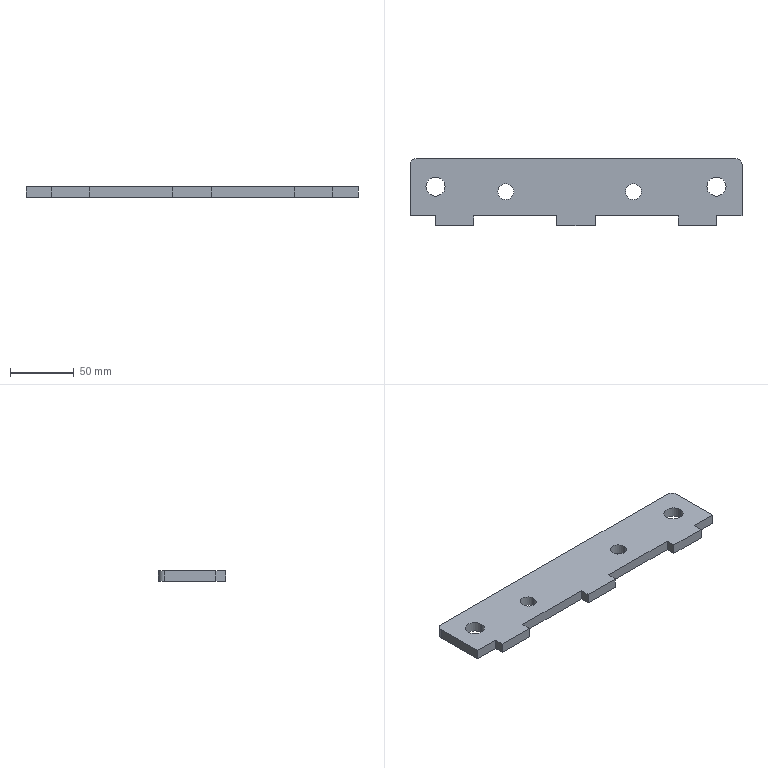Part | SolidWorks | features FlatPattern 1, SMBaseFlange 1, SheetMetal 1 | 1 solid | 28 faces | box 260 x 52.5 x 8 mm | volume 94123 mm3 | plane 18 | cylinder 10 | commonest cylinder face diameters 12.5 x4 15 x4 10 x2
STEP:
#1=CARTESIAN_POINT('',(-58.75,19.,8.));
#2=VERTEX_POINT('',#1);
#3=CARTESIAN_POINT('',(-46.25,19.,8.));
#4=VERTEX_POINT('',#3);
#5=CARTESIAN_POINT('',(-52.5,19.,8.));
#6=DIRECTION('',(0.,0.,1.));
#7=DIRECTION('',(1.,0.,0.));
#8=AXIS2_PLACEMENT_3D('',#5,#6,#7);
#9=CIRCLE('',#8,6.25);
#10=EDGE_CURVE('',#2,#4,#9,.T.);
#11=ORIENTED_EDGE('',*,*,#10,.T.);
#12=CARTESIAN_POINT('',(-46.25,19.,0.));
#13=VERTEX_POINT('',#12);
#14=CARTESIAN_POINT('',(-46.25,19.,8.));
#15=DIRECTION('',(0.,0.,-1.));
#16=VECTOR('',#15,1000.);
#17=LINE('',#14,#16);
#18=EDGE_CURVE('',#4,#13,#17,.T.);
#19=ORIENTED_EDGE('',*,*,#18,.T.);
#20=CARTESIAN_POINT('',(-58.75,19.,0.));
#21=VERTEX_POINT('',#20);
#22=CARTESIAN_POINT('',(-52.5,19.,0.));
#23=DIRECTION('',(0.,0.,1.));
#24=DIRECTION('',(1.,0.,0.));
#25=AXIS2_PLACEMENT_3D('',#22,#23,#24);
#26=CIRCLE('',#25,6.25);
#27=EDGE_CURVE('',#21,#13,#26,.T.);
#28=ORIENTED_EDGE('',*,*,#27,.F.);
#29=CARTESIAN_POINT('',(-58.75,19.,8.));
#30=DIRECTION('',(0.,0.,-1.));
#31=VECTOR('',#30,1000.);
#32=LINE('',#29,#31);
#33=EDGE_CURVE('',#2,#21,#32,.T.);
#34=ORIENTED_EDGE('',*,*,#33,.F.);
#35=EDGE_LOOP('',(#11,#19,#28,#34));
#36=FACE_OUTER_BOUND('',#35,.T.);
#37=CARTESIAN_POINT('',(-52.5,19.,8.));
#38=DIRECTION('',(0.,0.,-1.));
#39=DIRECTION('',(-1.,0.,0.));
#40=AXIS2_PLACEMENT_3D('',#37,#38,#39);
#41=CYLINDRICAL_SURFACE('',#40,6.25);
#42=ADVANCED_FACE('',(#36),#41,.F.);
#43=CARTESIAN_POINT('',(41.25,19.,8.));
#44=VERTEX_POINT('',#43);
#45=CARTESIAN_POINT('',(53.75,19.,8.));
#46=VERTEX_POINT('',#45);
#47=CARTESIAN_POINT('',(47.5,19.,8.));
#48=DIRECTION('',(0.,0.,1.));
#49=DIRECTION('',(1.,0.,0.));
#50=AXIS2_PLACEMENT_3D('',#47,#48,#49);
#51=CIRCLE('',#50,6.25);
#52=EDGE_CURVE('',#44,#46,#51,.T.);
#53=ORIENTED_EDGE('',*,*,#52,.T.);
#54=CARTESIAN_POINT('',(53.75,19.,0.));
#55=VERTEX_POINT('',#54);
#56=CARTESIAN_POINT('',(53.75,19.,8.));
#57=DIRECTION('',(0.,0.,-1.));
#58=VECTOR('',#57,1000.);
#59=LINE('',#56,#58);
#60=EDGE_CURVE('',#46,#55,#59,.T.);
#61=ORIENTED_EDGE('',*,*,#60,.T.);
#62=CARTESIAN_POINT('',(41.25,19.,0.));
#63=VERTEX_POINT('',#62);
#64=CARTESIAN_POINT('',(47.5,19.,0.));
#65=DIRECTION('',(0.,0.,1.));
#66=DIRECTION('',(1.,0.,0.));
#67=AXIS2_PLACEMENT_3D('',#64,#65,#66);
#68=CIRCLE('',#67,6.25);
#69=EDGE_CURVE('',#63,#55,#68,.T.);
#70=ORIENTED_EDGE('',*,*,#69,.F.);
#71=CARTESIAN_POINT('',(41.25,19.,8.));
#72=DIRECTION('',(0.,0.,-1.));
#73=VECTOR('',#72,1000.);
#74=LINE('',#71,#73);
#75=EDGE_CURVE('',#44,#63,#74,.T.);
#76=ORIENTED_EDGE('',*,*,#75,.F.);
#77=EDGE_LOOP('',(#53,#61,#70,#76));
#78=FACE_OUTER_BOUND('',#77,.T.);
#79=CARTESIAN_POINT('',(47.5,19.,8.));
#80=DIRECTION('',(0.,0.,-1.));
#81=DIRECTION('',(-1.,0.,0.));
#82=AXIS2_PLACEMENT_3D('',#79,#80,#81);
#83=CYLINDRICAL_SURFACE('',#82,6.25);
#84=ADVANCED_FACE('',(#78),#83,.F.);
#85=CARTESIAN_POINT('',(-115.,23.,8.));
#86=VERTEX_POINT('',#85);
#87=CARTESIAN_POINT('',(-100.,23.,8.));
#88=VERTEX_POINT('',#87);
#89=CARTESIAN_POINT('',(-107.5,23.,8.));
#90=DIRECTION('',(0.,0.,1.));
#91=DIRECTION('',(1.,0.,0.));
#92=AXIS2_PLACEMENT_3D('',#89,#90,#91);
#93=CIRCLE('',#92,7.5);
#94=EDGE_CURVE('',#86,#88,#93,.T.);
#95=ORIENTED_EDGE('',*,*,#94,.T.);
#96=CARTESIAN_POINT('',(-100.,23.,0.));
#97=VERTEX_POINT('',#96);
#98=CARTESIAN_POINT('',(-100.,23.,8.));
#99=DIRECTION('',(0.,0.,-1.));
#100=VECTOR('',#99,1000.);
#101=LINE('',#98,#100);
#102=EDGE_CURVE('',#88,#97,#101,.T.);
#103=ORIENTED_EDGE('',*,*,#102,.T.);
#104=CARTESIAN_POINT('',(-115.,23.,0.));
#105=VERTEX_POINT('',#104);
#106=CARTESIAN_POINT('',(-107.5,23.,0.));
#107=DIRECTION('',(0.,0.,1.));
#108=DIRECTION('',(1.,0.,0.));
#109=AXIS2_PLACEMENT_3D('',#106,#107,#108);
#110=CIRCLE('',#109,7.5);
#111=EDGE_CURVE('',#105,#97,#110,.T.);
#112=ORIENTED_EDGE('',*,*,#111,.F.);
#113=CARTESIAN_POINT('',(-115.,23.,8.));
#114=DIRECTION('',(0.,0.,-1.));
#115=VECTOR('',#114,1000.);
#116=LINE('',#113,#115);
#117=EDGE_CURVE('',#86,#105,#116,.T.);
#118=ORIENTED_EDGE('',*,*,#117,.F.);
#119=EDGE_LOOP('',(#95,#103,#112,#118));
#120=FACE_OUTER_BOUND('',#119,.T.);
#121=CARTESIAN_POINT('',(-107.5,23.,8.));
#122=DIRECTION('',(0.,0.,-1.));
#123=DIRECTION('',(-1.,0.,0.));
#124=AXIS2_PLACEMENT_3D('',#121,#122,#123);
#125=CYLINDRICAL_SURFACE('',#124,7.5);
#126=ADVANCED_FACE('',(#120),#125,.F.);
#127=CARTESIAN_POINT('',(105.,23.,8.));
#128=VERTEX_POINT('',#127);
#129=CARTESIAN_POINT('',(120.,23.,8.));
#130=VERTEX_POINT('',#129);
#131=CARTESIAN_POINT('',(112.5,23.,8.));
#132=DIRECTION('',(0.,0.,1.));
#133=DIRECTION('',(1.,0.,0.));
#134=AXIS2_PLACEMENT_3D('',#131,#132,#133);
#135=CIRCLE('',#134,7.5);
#136=EDGE_CURVE('',#128,#130,#135,.T.);
#137=ORIENTED_EDGE('',*,*,#136,.T.);
#138=CARTESIAN_POINT('',(120.,23.,0.));
#139=VERTEX_POINT('',#138);
#140=CARTESIAN_POINT('',(120.,23.,8.));
#141=DIRECTION('',(0.,0.,-1.));
#142=VECTOR('',#141,1000.);
#143=LINE('',#140,#142);
#144=EDGE_CURVE('',#130,#139,#143,.T.);
#145=ORIENTED_EDGE('',*,*,#144,.T.);
#146=CARTESIAN_POINT('',(105.,23.,0.));
#147=VERTEX_POINT('',#146);
#148=CARTESIAN_POINT('',(112.5,23.,0.));
#149=DIRECTION('',(0.,0.,1.));
#150=DIRECTION('',(1.,0.,0.));
#151=AXIS2_PLACEMENT_3D('',#148,#149,#150);
#152=CIRCLE('',#151,7.5);
#153=EDGE_CURVE('',#147,#139,#152,.T.);
#154=ORIENTED_EDGE('',*,*,#153,.F.);
#155=CARTESIAN_POINT('',(105.,23.,8.));
#156=DIRECTION('',(0.,0.,-1.));
#157=VECTOR('',#156,1000.);
#158=LINE('',#155,#157);
#159=EDGE_CURVE('',#128,#147,#158,.T.);
#160=ORIENTED_EDGE('',*,*,#159,.F.);
#161=EDGE_LOOP('',(#137,#145,#154,#160));
#162=FACE_OUTER_BOUND('',#161,.T.);
#163=CARTESIAN_POINT('',(112.5,23.,8.));
#164=DIRECTION('',(0.,0.,-1.));
#165=DIRECTION('',(-1.,0.,0.));
#166=AXIS2_PLACEMENT_3D('',#163,#164,#165);
#167=CYLINDRICAL_SURFACE('',#166,7.5);
#168=ADVANCED_FACE('',(#162),#167,.F.);
#169=ORIENTED_EDGE('',*,*,#52,.F.);
#170=CARTESIAN_POINT('',(47.5,19.,8.));
#171=DIRECTION('',(0.,0.,1.));
#172=DIRECTION('',(1.,0.,0.));
#173=AXIS2_PLACEMENT_3D('',#170,#171,#172);
#174=CIRCLE('',#173,6.25);
#175=EDGE_CURVE('',#46,#44,#174,.T.);
#176=ORIENTED_EDGE('',*,*,#175,.F.);
#177=EDGE_LOOP('',(#169,#176));
#178=FACE_BOUND('',#177,.T.);
#179=ORIENTED_EDGE('',*,*,#136,.F.);
#180=CARTESIAN_POINT('',(112.5,23.,8.));
#181=DIRECTION('',(0.,0.,1.));
#182=DIRECTION('',(1.,0.,0.));
#183=AXIS2_PLACEMENT_3D('',#180,#181,#182);
#184=CIRCLE('',#183,7.5);
#185=EDGE_CURVE('',#130,#128,#184,.T.);
#186=ORIENTED_EDGE('',*,*,#185,.F.);
#187=EDGE_LOOP('',(#179,#186));
#188=FACE_BOUND('',#187,.T.);
#189=CARTESIAN_POINT('',(112.5,0.,8.));
#190=VERTEX_POINT('',#189);
#191=CARTESIAN_POINT('',(132.5,0.,8.));
#192=VERTEX_POINT('',#191);
#193=CARTESIAN_POINT('',(112.5,0.,8.));
#194=DIRECTION('',(1.,0.,0.));
#195=VECTOR('',#194,1000.);
#196=LINE('',#193,#195);
#197=EDGE_CURVE('',#190,#192,#196,.T.);
#198=ORIENTED_EDGE('',*,*,#197,.T.);
#199=CARTESIAN_POINT('',(132.5,40.,8.));
#200=VERTEX_POINT('',#199);
#201=CARTESIAN_POINT('',(132.5,0.,8.));
#202=DIRECTION('',(0.,1.,0.));
#203=VECTOR('',#202,1000.);
#204=LINE('',#201,#203);
#205=EDGE_CURVE('',#192,#200,#204,.T.);
#206=ORIENTED_EDGE('',*,*,#205,.T.);
#207=CARTESIAN_POINT('',(127.5,45.,8.));
#208=VERTEX_POINT('',#207);
#209=CARTESIAN_POINT('',(127.5,40.,8.));
#210=DIRECTION('',(0.,0.,1.));
#211=DIRECTION('',(1.,0.,0.));
#212=AXIS2_PLACEMENT_3D('',#209,#210,#211);
#213=CIRCLE('',#212,5.);
#214=EDGE_CURVE('',#200,#208,#213,.T.);
#215=ORIENTED_EDGE('',*,*,#214,.T.);
#216=CARTESIAN_POINT('',(-122.5,45.,8.));
#217=VERTEX_POINT('',#216);
#218=CARTESIAN_POINT('',(127.5,45.,8.));
#219=DIRECTION('',(-1.,0.,0.));
#220=VECTOR('',#219,1000.);
#221=LINE('',#218,#220);
#222=EDGE_CURVE('',#208,#217,#221,.T.);
#223=ORIENTED_EDGE('',*,*,#222,.T.);
#224=CARTESIAN_POINT('',(-127.5,40.,8.));
#225=VERTEX_POINT('',#224);
#226=CARTESIAN_POINT('',(-122.5,40.,8.));
#227=DIRECTION('',(0.,0.,1.));
#228=DIRECTION('',(1.,0.,0.));
#229=AXIS2_PLACEMENT_3D('',#226,#227,#228);
#230=CIRCLE('',#229,5.);
#231=EDGE_CURVE('',#217,#225,#230,.T.);
#232=ORIENTED_EDGE('',*,*,#231,.T.);
#233=CARTESIAN_POINT('',(-127.5,0.,8.));
#234=VERTEX_POINT('',#233);
#235=CARTESIAN_POINT('',(-127.5,40.,8.));
#236=DIRECTION('',(0.,-1.,0.));
#237=VECTOR('',#236,1000.);
#238=LINE('',#235,#237);
#239=EDGE_CURVE('',#225,#234,#238,.T.);
#240=ORIENTED_EDGE('',*,*,#239,.T.);
#241=CARTESIAN_POINT('',(-107.5,0.,8.));
#242=VERTEX_POINT('',#241);
#243=CARTESIAN_POINT('',(-127.5,0.,8.));
#244=DIRECTION('',(1.,0.,0.));
#245=VECTOR('',#244,1000.);
#246=LINE('',#243,#245);
#247=EDGE_CURVE('',#234,#242,#246,.T.);
#248=ORIENTED_EDGE('',*,*,#247,.T.);
#249=CARTESIAN_POINT('',(-107.5,-7.5,8.));
#250=VERTEX_POINT('',#249);
#251=CARTESIAN_POINT('',(-107.5,0.,8.));
#252=DIRECTION('',(0.,-1.,0.));
#253=VECTOR('',#252,1000.);
#254=LINE('',#251,#253);
#255=EDGE_CURVE('',#242,#250,#254,.T.);
#256=ORIENTED_EDGE('',*,*,#255,.T.);
#257=CARTESIAN_POINT('',(-77.5,-7.5,8.));
#258=VERTEX_POINT('',#257);
#259=CARTESIAN_POINT('',(-107.5,-7.5,8.));
#260=DIRECTION('',(1.,0.,0.));
#261=VECTOR('',#260,1000.);
#262=LINE('',#259,#261);
#263=EDGE_CURVE('',#250,#258,#262,.T.);
#264=ORIENTED_EDGE('',*,*,#263,.T.);
#265=CARTESIAN_POINT('',(-77.5,0.,8.));
#266=VERTEX_POINT('',#265);
#267=CARTESIAN_POINT('',(-77.5,-7.5,8.));
#268=DIRECTION('',(0.,1.,0.));
#269=VECTOR('',#268,1000.);
#270=LINE('',#267,#269);
#271=EDGE_CURVE('',#258,#266,#270,.T.);
#272=ORIENTED_EDGE('',*,*,#271,.T.);
#273=CARTESIAN_POINT('',(-12.5,0.,8.));
#274=VERTEX_POINT('',#273);
#275=CARTESIAN_POINT('',(-77.5,0.,8.));
#276=DIRECTION('',(1.,0.,0.));
#277=VECTOR('',#276,1000.);
#278=LINE('',#275,#277);
#279=EDGE_CURVE('',#266,#274,#278,.T.);
#280=ORIENTED_EDGE('',*,*,#279,.T.);
#281=CARTESIAN_POINT('',(-12.5,-7.5,8.));
#282=VERTEX_POINT('',#281);
#283=CARTESIAN_POINT('',(-12.5,0.,8.));
#284=DIRECTION('',(0.,-1.,0.));
#285=VECTOR('',#284,1000.);
#286=LINE('',#283,#285);
#287=EDGE_CURVE('',#274,#282,#286,.T.);
#288=ORIENTED_EDGE('',*,*,#287,.T.);
#289=CARTESIAN_POINT('',(17.5,-7.5,8.));
#290=VERTEX_POINT('',#289);
#291=CARTESIAN_POINT('',(-12.5,-7.5,8.));
#292=DIRECTION('',(1.,0.,0.));
#293=VECTOR('',#292,1000.);
#294=LINE('',#291,#293);
#295=EDGE_CURVE('',#282,#290,#294,.T.);
#296=ORIENTED_EDGE('',*,*,#295,.T.);
#297=CARTESIAN_POINT('',(17.5,0.,8.));
#298=VERTEX_POINT('',#297);
#299=CARTESIAN_POINT('',(17.5,-7.5,8.));
#300=DIRECTION('',(0.,1.,0.));
#301=VECTOR('',#300,1000.);
#302=LINE('',#299,#301);
#303=EDGE_CURVE('',#290,#298,#302,.T.);
#304=ORIENTED_EDGE('',*,*,#303,.T.);
#305=CARTESIAN_POINT('',(82.5,0.,8.));
#306=VERTEX_POINT('',#305);
#307=CARTESIAN_POINT('',(17.5,0.,8.));
#308=DIRECTION('',(1.,0.,0.));
#309=VECTOR('',#308,1000.);
#310=LINE('',#307,#309);
#311=EDGE_CURVE('',#298,#306,#310,.T.);
#312=ORIENTED_EDGE('',*,*,#311,.T.);
#313=CARTESIAN_POINT('',(82.5,-7.5,8.));
#314=VERTEX_POINT('',#313);
#315=CARTESIAN_POINT('',(82.5,0.,8.));
#316=DIRECTION('',(0.,-1.,0.));
#317=VECTOR('',#316,1000.);
#318=LINE('',#315,#317);
#319=EDGE_CURVE('',#306,#314,#318,.T.);
#320=ORIENTED_EDGE('',*,*,#319,.T.);
#321=CARTESIAN_POINT('',(112.5,-7.5,8.));
#322=VERTEX_POINT('',#321);
#323=CARTESIAN_POINT('',(82.5,-7.5,8.));
#324=DIRECTION('',(1.,0.,0.));
#325=VECTOR('',#324,1000.);
#326=LINE('',#323,#325);
#327=EDGE_CURVE('',#314,#322,#326,.T.);
#328=ORIENTED_EDGE('',*,*,#327,.T.);
#329=CARTESIAN_POINT('',(112.5,-7.5,8.));
#330=DIRECTION('',(0.,1.,0.));
#331=VECTOR('',#330,1000.);
#332=LINE('',#329,#331);
#333=EDGE_CURVE('',#322,#190,#332,.T.);
#334=ORIENTED_EDGE('',*,*,#333,.T.);
#335=EDGE_LOOP('',(#198,#206,#215,#223,#232,#240,#248,#256,#264,#272,#280,#288,#296,#304,#312,#320,#328,#334));
#336=FACE_OUTER_BOUND('',#335,.T.);
#337=ORIENTED_EDGE('',*,*,#94,.F.);
#338=CARTESIAN_POINT('',(-107.5,23.,8.));
#339=DIRECTION('',(0.,0.,1.));
#340=DIRECTION('',(1.,0.,0.));
#341=AXIS2_PLACEMENT_3D('',#338,#339,#340);
#342=CIRCLE('',#341,7.5);
#343=EDGE_CURVE('',#88,#86,#342,.T.);
#344=ORIENTED_EDGE('',*,*,#343,.F.);
#345=EDGE_LOOP('',(#337,#344));
#346=FACE_BOUND('',#345,.T.);
#347=ORIENTED_EDGE('',*,*,#10,.F.);
#348=CARTESIAN_POINT('',(-52.5,19.,8.));
#349=DIRECTION('',(0.,0.,1.));
#350=DIRECTION('',(1.,0.,0.));
#351=AXIS2_PLACEMENT_3D('',#348,#349,#350);
#352=CIRCLE('',#351,6.25);
#353=EDGE_CURVE('',#4,#2,#352,.T.);
#354=ORIENTED_EDGE('',*,*,#353,.F.);
#355=EDGE_LOOP('',(#347,#354));
#356=FACE_BOUND('',#355,.T.);
#357=CARTESIAN_POINT('',(127.5,40.,8.));
#358=DIRECTION('',(0.,0.,1.));
#359=DIRECTION('',(1.,0.,0.));
#360=AXIS2_PLACEMENT_3D('',#357,#358,#359);
#361=PLANE('',#360);
#362=ADVANCED_FACE('',(#178,#188,#336,#346,#356),#361,.T.);
#363=CARTESIAN_POINT('',(112.5,0.,0.));
#364=VERTEX_POINT('',#363);
#365=CARTESIAN_POINT('',(132.5,0.,0.));
#366=VERTEX_POINT('',#365);
#367=CARTESIAN_POINT('',(112.5,0.,0.));
#368=DIRECTION('',(1.,0.,0.));
#369=VECTOR('',#368,1000.);
#370=LINE('',#367,#369);
#371=EDGE_CURVE('',#364,#366,#370,.T.);
#372=ORIENTED_EDGE('',*,*,#371,.F.);
#373=CARTESIAN_POINT('',(112.5,-7.5,0.));
#374=VERTEX_POINT('',#373);
#375=CARTESIAN_POINT('',(112.5,-7.5,0.));
#376=DIRECTION('',(0.,1.,0.));
#377=VECTOR('',#376,1000.);
#378=LINE('',#375,#377);
#379=EDGE_CURVE('',#374,#364,#378,.T.);
#380=ORIENTED_EDGE('',*,*,#379,.F.);
#381=CARTESIAN_POINT('',(82.5,-7.5,0.));
#382=VERTEX_POINT('',#381);
#383=CARTESIAN_POINT('',(82.5,-7.5,0.));
#384=DIRECTION('',(1.,0.,0.));
#385=VECTOR('',#384,1000.);
#386=LINE('',#383,#385);
#387=EDGE_CURVE('',#382,#374,#386,.T.);
#388=ORIENTED_EDGE('',*,*,#387,.F.);
#389=CARTESIAN_POINT('',(82.5,0.,0.));
#390=VERTEX_POINT('',#389);
#391=CARTESIAN_POINT('',(82.5,0.,0.));
#392=DIRECTION('',(0.,-1.,0.));
#393=VECTOR('',#392,1000.);
#394=LINE('',#391,#393);
#395=EDGE_CURVE('',#390,#382,#394,.T.);
#396=ORIENTED_EDGE('',*,*,#395,.F.);
#397=CARTESIAN_POINT('',(17.5,0.,0.));
#398=VERTEX_POINT('',#397);
#399=CARTESIAN_POINT('',(17.5,0.,0.));
#400=DIRECTION('',(1.,0.,0.));
#401=VECTOR('',#400,1000.);
#402=LINE('',#399,#401);
#403=EDGE_CURVE('',#398,#390,#402,.T.);
#404=ORIENTED_EDGE('',*,*,#403,.F.);
#405=CARTESIAN_POINT('',(17.5,-7.5,0.));
#406=VERTEX_POINT('',#405);
#407=CARTESIAN_POINT('',(17.5,-7.5,0.));
#408=DIRECTION('',(0.,1.,0.));
#409=VECTOR('',#408,1000.);
#410=LINE('',#407,#409);
#411=EDGE_CURVE('',#406,#398,#410,.T.);
#412=ORIENTED_EDGE('',*,*,#411,.F.);
#413=CARTESIAN_POINT('',(-12.5,-7.5,0.));
#414=VERTEX_POINT('',#413);
#415=CARTESIAN_POINT('',(-12.5,-7.5,0.));
#416=DIRECTION('',(1.,0.,0.));
#417=VECTOR('',#416,1000.);
#418=LINE('',#415,#417);
#419=EDGE_CURVE('',#414,#406,#418,.T.);
#420=ORIENTED_EDGE('',*,*,#419,.F.);
#421=CARTESIAN_POINT('',(-12.5,0.,0.));
#422=VERTEX_POINT('',#421);
#423=CARTESIAN_POINT('',(-12.5,0.,0.));
#424=DIRECTION('',(0.,-1.,0.));
#425=VECTOR('',#424,1000.);
#426=LINE('',#423,#425);
#427=EDGE_CURVE('',#422,#414,#426,.T.);
#428=ORIENTED_EDGE('',*,*,#427,.F.);
#429=CARTESIAN_POINT('',(-77.5,0.,0.));
#430=VERTEX_POINT('',#429);
#431=CARTESIAN_POINT('',(-77.5,0.,0.));
#432=DIRECTION('',(1.,0.,0.));
#433=VECTOR('',#432,1000.);
#434=LINE('',#431,#433);
#435=EDGE_CURVE('',#430,#422,#434,.T.);
#436=ORIENTED_EDGE('',*,*,#435,.F.);
#437=CARTESIAN_POINT('',(-77.5,-7.5,0.));
#438=VERTEX_POINT('',#437);
#439=CARTESIAN_POINT('',(-77.5,-7.5,0.));
#440=DIRECTION('',(0.,1.,0.));
#441=VECTOR('',#440,1000.);
#442=LINE('',#439,#441);
#443=EDGE_CURVE('',#438,#430,#442,.T.);
#444=ORIENTED_EDGE('',*,*,#443,.F.);
#445=CARTESIAN_POINT('',(-107.5,-7.5,0.));
#446=VERTEX_POINT('',#445);
#447=CARTESIAN_POINT('',(-107.5,-7.5,0.));
#448=DIRECTION('',(1.,0.,0.));
#449=VECTOR('',#448,1000.);
#450=LINE('',#447,#449);
#451=EDGE_CURVE('',#446,#438,#450,.T.);
#452=ORIENTED_EDGE('',*,*,#451,.F.);
#453=CARTESIAN_POINT('',(-107.5,0.,0.));
#454=VERTEX_POINT('',#453);
#455=CARTESIAN_POINT('',(-107.5,0.,0.));
#456=DIRECTION('',(0.,-1.,0.));
#457=VECTOR('',#456,1000.);
#458=LINE('',#455,#457);
#459=EDGE_CURVE('',#454,#446,#458,.T.);
#460=ORIENTED_EDGE('',*,*,#459,.F.);
#461=CARTESIAN_POINT('',(-127.5,0.,0.));
#462=VERTEX_POINT('',#461);
#463=CARTESIAN_POINT('',(-127.5,0.,0.));
#464=DIRECTION('',(1.,0.,0.));
#465=VECTOR('',#464,1000.);
#466=LINE('',#463,#465);
#467=EDGE_CURVE('',#462,#454,#466,.T.);
#468=ORIENTED_EDGE('',*,*,#467,.F.);
#469=CARTESIAN_POINT('',(-127.5,40.,0.));
#470=VERTEX_POINT('',#469);
#471=CARTESIAN_POINT('',(-127.5,40.,0.));
#472=DIRECTION('',(0.,-1.,0.));
#473=VECTOR('',#472,1000.);
#474=LINE('',#471,#473);
#475=EDGE_CURVE('',#470,#462,#474,.T.);
#476=ORIENTED_EDGE('',*,*,#475,.F.);
#477=CARTESIAN_POINT('',(-122.5,45.,0.));
#478=VERTEX_POINT('',#477);
#479=CARTESIAN_POINT('',(-122.5,40.,0.));
#480=DIRECTION('',(0.,0.,1.));
#481=DIRECTION('',(1.,0.,0.));
#482=AXIS2_PLACEMENT_3D('',#479,#480,#481);
#483=CIRCLE('',#482,5.);
#484=EDGE_CURVE('',#478,#470,#483,.T.);
#485=ORIENTED_EDGE('',*,*,#484,.F.);
#486=CARTESIAN_POINT('',(127.5,45.,0.));
#487=VERTEX_POINT('',#486);
#488=CARTESIAN_POINT('',(127.5,45.,0.));
#489=DIRECTION('',(-1.,0.,0.));
#490=VECTOR('',#489,1000.);
#491=LINE('',#488,#490);
#492=EDGE_CURVE('',#487,#478,#491,.T.);
#493=ORIENTED_EDGE('',*,*,#492,.F.);
#494=CARTESIAN_POINT('',(132.5,40.,0.));
#495=VERTEX_POINT('',#494);
#496=CARTESIAN_POINT('',(127.5,40.,0.));
#497=DIRECTION('',(0.,0.,1.));
#498=DIRECTION('',(1.,0.,0.));
#499=AXIS2_PLACEMENT_3D('',#496,#497,#498);
#500=CIRCLE('',#499,5.);
#501=EDGE_CURVE('',#495,#487,#500,.T.);
#502=ORIENTED_EDGE('',*,*,#501,.F.);
#503=CARTESIAN_POINT('',(132.5,0.,0.));
#504=DIRECTION('',(0.,1.,0.));
#505=VECTOR('',#504,1000.);
#506=LINE('',#503,#505);
#507=EDGE_CURVE('',#366,#495,#506,.T.);
#508=ORIENTED_EDGE('',*,*,#507,.F.);
#509=EDGE_LOOP('',(#372,#380,#388,#396,#404,#412,#420,#428,#436,#444,#452,#460,#468,#476,#485,#493,#502,#508));
#510=FACE_OUTER_BOUND('',#509,.T.);
#511=ORIENTED_EDGE('',*,*,#153,.T.);
#512=CARTESIAN_POINT('',(112.5,23.,0.));
#513=DIRECTION('',(0.,0.,1.));
#514=DIRECTION('',(1.,0.,0.));
#515=AXIS2_PLACEMENT_3D('',#512,#513,#514);
#516=CIRCLE('',#515,7.5);
#517=EDGE_CURVE('',#139,#147,#516,.T.);
#518=ORIENTED_EDGE('',*,*,#517,.T.);
#519=EDGE_LOOP('',(#511,#518));
#520=FACE_BOUND('',#519,.T.);
#521=ORIENTED_EDGE('',*,*,#111,.T.);
#522=CARTESIAN_POINT('',(-107.5,23.,0.));
#523=DIRECTION('',(0.,0.,1.));
#524=DIRECTION('',(1.,0.,0.));
#525=AXIS2_PLACEMENT_3D('',#522,#523,#524);
#526=CIRCLE('',#525,7.5);
#527=EDGE_CURVE('',#97,#105,#526,.T.);
#528=ORIENTED_EDGE('',*,*,#527,.T.);
#529=EDGE_LOOP('',(#521,#528));
#530=FACE_BOUND('',#529,.T.);
#531=ORIENTED_EDGE('',*,*,#69,.T.);
#532=CARTESIAN_POINT('',(47.5,19.,0.));
#533=DIRECTION('',(0.,0.,1.));
#534=DIRECTION('',(1.,0.,0.));
#535=AXIS2_PLACEMENT_3D('',#532,#533,#534);
#536=CIRCLE('',#535,6.25);
#537=EDGE_CURVE('',#55,#63,#536,.T.);
#538=ORIENTED_EDGE('',*,*,#537,.T.);
#539=EDGE_LOOP('',(#531,#538));
#540=FACE_BOUND('',#539,.T.);
#541=ORIENTED_EDGE('',*,*,#27,.T.);
#542=CARTESIAN_POINT('',(-52.5,19.,0.));
#543=DIRECTION('',(0.,0.,1.));
#544=DIRECTION('',(1.,0.,0.));
#545=AXIS2_PLACEMENT_3D('',#542,#543,#544);
#546=CIRCLE('',#545,6.25);
#547=EDGE_CURVE('',#13,#21,#546,.T.);
#548=ORIENTED_EDGE('',*,*,#547,.T.);
#549=EDGE_LOOP('',(#541,#548));
#550=FACE_BOUND('',#549,.T.);
#551=CARTESIAN_POINT('',(127.5,40.,0.));
#552=DIRECTION('',(0.,0.,1.));
#553=DIRECTION('',(1.,0.,0.));
#554=AXIS2_PLACEMENT_3D('',#551,#552,#553);
#555=PLANE('',#554);
#556=ADVANCED_FACE('',(#510,#520,#530,#540,#550),#555,.F.);
#557=ORIENTED_EDGE('',*,*,#371,.T.);
#558=CARTESIAN_POINT('',(132.5,0.,8.));
#559=DIRECTION('',(0.,0.,-1.));
#560=VECTOR('',#559,1000.);
#561=LINE('',#558,#560);
#562=EDGE_CURVE('',#192,#366,#561,.T.);
#563=ORIENTED_EDGE('',*,*,#562,.F.);
#564=ORIENTED_EDGE('',*,*,#197,.F.);
#565=CARTESIAN_POINT('',(112.5,0.,8.));
#566=DIRECTION('',(0.,0.,-1.));
#567=VECTOR('',#566,1000.);
#568=LINE('',#565,#567);
#569=EDGE_CURVE('',#190,#364,#568,.T.);
#570=ORIENTED_EDGE('',*,*,#569,.T.);
#571=EDGE_LOOP('',(#557,#563,#564,#570));
#572=FACE_OUTER_BOUND('',#571,.T.);
#573=CARTESIAN_POINT('',(112.5,0.,8.));
#574=DIRECTION('',(0.,1.,0.));
#575=DIRECTION('',(0.,0.,1.));
#576=AXIS2_PLACEMENT_3D('',#573,#574,#575);
#577=PLANE('',#576);
#578=ADVANCED_FACE('',(#572),#577,.F.);
#579=ORIENTED_EDGE('',*,*,#507,.T.);
#580=CARTESIAN_POINT('',(132.5,40.,8.));
#581=DIRECTION('',(0.,0.,-1.));
#582=VECTOR('',#581,1000.);
#583=LINE('',#580,#582);
#584=EDGE_CURVE('',#200,#495,#583,.T.);
#585=ORIENTED_EDGE('',*,*,#584,.F.);
#586=ORIENTED_EDGE('',*,*,#205,.F.);
#587=ORIENTED_EDGE('',*,*,#562,.T.);
#588=EDGE_LOOP('',(#579,#585,#586,#587));
#589=FACE_OUTER_BOUND('',#588,.T.);
#590=CARTESIAN_POINT('',(132.5,0.,8.));
#591=DIRECTION('',(-1.,0.,0.));
#592=DIRECTION('',(0.,0.,1.));
#593=AXIS2_PLACEMENT_3D('',#590,#591,#592);
#594=PLANE('',#593);
#595=ADVANCED_FACE('',(#589),#594,.F.);
#596=ORIENTED_EDGE('',*,*,#501,.T.);
#597=CARTESIAN_POINT('',(127.5,45.,8.));
#598=DIRECTION('',(0.,0.,-1.));
#599=VECTOR('',#598,1000.);
#600=LINE('',#597,#599);
#601=EDGE_CURVE('',#208,#487,#600,.T.);
#602=ORIENTED_EDGE('',*,*,#601,.F.);
#603=ORIENTED_EDGE('',*,*,#214,.F.);
#604=ORIENTED_EDGE('',*,*,#584,.T.);
#605=EDGE_LOOP('',(#596,#602,#603,#604));
#606=FACE_OUTER_BOUND('',#605,.T.);
#607=CARTESIAN_POINT('',(127.5,40.,8.));
#608=DIRECTION('',(0.,0.,-1.));
#609=DIRECTION('',(-1.,0.,0.));
#610=AXIS2_PLACEMENT_3D('',#607,#608,#609);
#611=CYLINDRICAL_SURFACE('',#610,5.);
#612=ADVANCED_FACE('',(#606),#611,.T.);
#613=ORIENTED_EDGE('',*,*,#492,.T.);
#614=CARTESIAN_POINT('',(-122.5,45.,8.));
#615=DIRECTION('',(0.,0.,-1.));
#616=VECTOR('',#615,1000.);
#617=LINE('',#614,#616);
#618=EDGE_CURVE('',#217,#478,#617,.T.);
#619=ORIENTED_EDGE('',*,*,#618,.F.);
#620=ORIENTED_EDGE('',*,*,#222,.F.);
#621=ORIENTED_EDGE('',*,*,#601,.T.);
#622=EDGE_LOOP('',(#613,#619,#620,#621));
#623=FACE_OUTER_BOUND('',#622,.T.);
#624=CARTESIAN_POINT('',(127.5,45.,8.));
#625=DIRECTION('',(0.,-1.,0.));
#626=DIRECTION('',(1.,0.,0.));
#627=AXIS2_PLACEMENT_3D('',#624,#625,#626);
#628=PLANE('',#627);
#629=ADVANCED_FACE('',(#623),#628,.F.);
#630=ORIENTED_EDGE('',*,*,#484,.T.);
#631=CARTESIAN_POINT('',(-127.5,40.,8.));
#632=DIRECTION('',(0.,0.,-1.));
#633=VECTOR('',#632,1000.);
#634=LINE('',#631,#633);
#635=EDGE_CURVE('',#225,#470,#634,.T.);
#636=ORIENTED_EDGE('',*,*,#635,.F.);
#637=ORIENTED_EDGE('',*,*,#231,.F.);
#638=ORIENTED_EDGE('',*,*,#618,.T.);
#639=EDGE_LOOP('',(#630,#636,#637,#638));
#640=FACE_OUTER_BOUND('',#639,.T.);
#641=CARTESIAN_POINT('',(-122.5,40.,8.));
#642=DIRECTION('',(0.,0.,-1.));
#643=DIRECTION('',(-1.,0.,0.));
#644=AXIS2_PLACEMENT_3D('',#641,#642,#643);
#645=CYLINDRICAL_SURFACE('',#644,5.);
#646=ADVANCED_FACE('',(#640),#645,.T.);
#647=ORIENTED_EDGE('',*,*,#475,.T.);
#648=CARTESIAN_POINT('',(-127.5,0.,8.));
#649=DIRECTION('',(0.,0.,-1.));
#650=VECTOR('',#649,1000.);
#651=LINE('',#648,#650);
#652=EDGE_CURVE('',#234,#462,#651,.T.);
#653=ORIENTED_EDGE('',*,*,#652,.F.);
#654=ORIENTED_EDGE('',*,*,#239,.F.);
#655=ORIENTED_EDGE('',*,*,#635,.T.);
#656=EDGE_LOOP('',(#647,#653,#654,#655));
#657=FACE_OUTER_BOUND('',#656,.T.);
#658=CARTESIAN_POINT('',(-127.5,40.,8.));
#659=DIRECTION('',(1.,0.,0.));
#660=DIRECTION('',(0.,0.,-1.));
#661=AXIS2_PLACEMENT_3D('',#658,#659,#660);
#662=PLANE('',#661);
#663=ADVANCED_FACE('',(#657),#662,.F.);
#664=ORIENTED_EDGE('',*,*,#467,.T.);
#665=CARTESIAN_POINT('',(-107.5,0.,8.));
#666=DIRECTION('',(0.,0.,-1.));
#667=VECTOR('',#666,1000.);
#668=LINE('',#665,#667);
#669=EDGE_CURVE('',#242,#454,#668,.T.);
#670=ORIENTED_EDGE('',*,*,#669,.F.);
#671=ORIENTED_EDGE('',*,*,#247,.F.);
#672=ORIENTED_EDGE('',*,*,#652,.T.);
#673=EDGE_LOOP('',(#664,#670,#671,#672));
#674=FACE_OUTER_BOUND('',#673,.T.);
#675=CARTESIAN_POINT('',(-127.5,0.,8.));
#676=DIRECTION('',(0.,1.,0.));
#677=DIRECTION('',(-1.,0.,0.));
#678=AXIS2_PLACEMENT_3D('',#675,#676,#677);
#679=PLANE('',#678);
#680=ADVANCED_FACE('',(#674),#679,.F.);
#681=ORIENTED_EDGE('',*,*,#459,.T.);
#682=CARTESIAN_POINT('',(-107.5,-7.5,8.));
#683=DIRECTION('',(0.,0.,-1.));
#684=VECTOR('',#683,1000.);
#685=LINE('',#682,#684);
#686=EDGE_CURVE('',#250,#446,#685,.T.);
#687=ORIENTED_EDGE('',*,*,#686,.F.);
#688=ORIENTED_EDGE('',*,*,#255,.F.);
#689=ORIENTED_EDGE('',*,*,#669,.T.);
#690=EDGE_LOOP('',(#681,#687,#688,#689));
#691=FACE_OUTER_BOUND('',#690,.T.);
#692=CARTESIAN_POINT('',(-107.5,0.,8.));
#693=DIRECTION('',(1.,0.,0.));
#694=DIRECTION('',(0.,0.,-1.));
#695=AXIS2_PLACEMENT_3D('',#692,#693,#694);
#696=PLANE('',#695);
#697=ADVANCED_FACE('',(#691),#696,.F.);
#698=ORIENTED_EDGE('',*,*,#451,.T.);
#699=CARTESIAN_POINT('',(-77.5,-7.5,8.));
#700=DIRECTION('',(0.,0.,-1.));
#701=VECTOR('',#700,1000.);
#702=LINE('',#699,#701);
#703=EDGE_CURVE('',#258,#438,#702,.T.);
#704=ORIENTED_EDGE('',*,*,#703,.F.);
#705=ORIENTED_EDGE('',*,*,#263,.F.);
#706=ORIENTED_EDGE('',*,*,#686,.T.);
#707=EDGE_LOOP('',(#698,#704,#705,#706));
#708=FACE_OUTER_BOUND('',#707,.T.);
#709=CARTESIAN_POINT('',(-107.5,-7.5,8.));
#710=DIRECTION('',(0.,1.,0.));
#711=DIRECTION('',(0.,0.,1.));
#712=AXIS2_PLACEMENT_3D('',#709,#710,#711);
#713=PLANE('',#712);
#714=ADVANCED_FACE('',(#708),#713,.F.);
#715=ORIENTED_EDGE('',*,*,#443,.T.);
#716=CARTESIAN_POINT('',(-77.5,0.,8.));
#717=DIRECTION('',(0.,0.,-1.));
#718=VECTOR('',#717,1000.);
#719=LINE('',#716,#718);
#720=EDGE_CURVE('',#266,#430,#719,.T.);
#721=ORIENTED_EDGE('',*,*,#720,.F.);
#722=ORIENTED_EDGE('',*,*,#271,.F.);
#723=ORIENTED_EDGE('',*,*,#703,.T.);
#724=EDGE_LOOP('',(#715,#721,#722,#723));
#725=FACE_OUTER_BOUND('',#724,.T.);
#726=CARTESIAN_POINT('',(-77.5,-7.5,8.));
#727=DIRECTION('',(-1.,0.,0.));
#728=DIRECTION('',(0.,0.,1.));
#729=AXIS2_PLACEMENT_3D('',#726,#727,#728);
#730=PLANE('',#729);
#731=ADVANCED_FACE('',(#725),#730,.F.);
#732=ORIENTED_EDGE('',*,*,#435,.T.);
#733=CARTESIAN_POINT('',(-12.5,0.,8.));
#734=DIRECTION('',(0.,0.,-1.));
#735=VECTOR('',#734,1000.);
#736=LINE('',#733,#735);
#737=EDGE_CURVE('',#274,#422,#736,.T.);
#738=ORIENTED_EDGE('',*,*,#737,.F.);
#739=ORIENTED_EDGE('',*,*,#279,.F.);
#740=ORIENTED_EDGE('',*,*,#720,.T.);
#741=EDGE_LOOP('',(#732,#738,#739,#740));
#742=FACE_OUTER_BOUND('',#741,.T.);
#743=CARTESIAN_POINT('',(-77.5,0.,8.));
#744=DIRECTION('',(0.,1.,0.));
#745=DIRECTION('',(-1.,0.,0.));
#746=AXIS2_PLACEMENT_3D('',#743,#744,#745);
#747=PLANE('',#746);
#748=ADVANCED_FACE('',(#742),#747,.F.);
#749=ORIENTED_EDGE('',*,*,#427,.T.);
#750=CARTESIAN_POINT('',(-12.5,-7.5,8.));
#751=DIRECTION('',(0.,0.,-1.));
#752=VECTOR('',#751,1000.);
#753=LINE('',#750,#752);
#754=EDGE_CURVE('',#282,#414,#753,.T.);
#755=ORIENTED_EDGE('',*,*,#754,.F.);
#756=ORIENTED_EDGE('',*,*,#287,.F.);
#757=ORIENTED_EDGE('',*,*,#737,.T.);
#758=EDGE_LOOP('',(#749,#755,#756,#757));
#759=FACE_OUTER_BOUND('',#758,.T.);
#760=CARTESIAN_POINT('',(-12.5,0.,8.));
#761=DIRECTION('',(1.,0.,0.));
#762=DIRECTION('',(0.,1.,0.));
#763=AXIS2_PLACEMENT_3D('',#760,#761,#762);
#764=PLANE('',#763);
#765=ADVANCED_FACE('',(#759),#764,.F.);
#766=ORIENTED_EDGE('',*,*,#419,.T.);
#767=CARTESIAN_POINT('',(17.5,-7.5,8.));
#768=DIRECTION('',(0.,0.,-1.));
#769=VECTOR('',#768,1000.);
#770=LINE('',#767,#769);
#771=EDGE_CURVE('',#290,#406,#770,.T.);
#772=ORIENTED_EDGE('',*,*,#771,.F.);
#773=ORIENTED_EDGE('',*,*,#295,.F.);
#774=ORIENTED_EDGE('',*,*,#754,.T.);
#775=EDGE_LOOP('',(#766,#772,#773,#774));
#776=FACE_OUTER_BOUND('',#775,.T.);
#777=CARTESIAN_POINT('',(-12.5,-7.5,8.));
#778=DIRECTION('',(0.,1.,0.));
#779=DIRECTION('',(0.,0.,1.));
#780=AXIS2_PLACEMENT_3D('',#777,#778,#779);
#781=PLANE('',#780);
#782=ADVANCED_FACE('',(#776),#781,.F.);
#783=ORIENTED_EDGE('',*,*,#411,.T.);
#784=CARTESIAN_POINT('',(17.5,0.,8.));
#785=DIRECTION('',(0.,0.,-1.));
#786=VECTOR('',#785,1000.);
#787=LINE('',#784,#786);
#788=EDGE_CURVE('',#298,#398,#787,.T.);
#789=ORIENTED_EDGE('',*,*,#788,.F.);
#790=ORIENTED_EDGE('',*,*,#303,.F.);
#791=ORIENTED_EDGE('',*,*,#771,.T.);
#792=EDGE_LOOP('',(#783,#789,#790,#791));
#793=FACE_OUTER_BOUND('',#792,.T.);
#794=CARTESIAN_POINT('',(17.5,-7.5,8.));
#795=DIRECTION('',(-1.,0.,0.));
#796=DIRECTION('',(0.,0.,1.));
#797=AXIS2_PLACEMENT_3D('',#794,#795,#796);
#798=PLANE('',#797);
#799=ADVANCED_FACE('',(#793),#798,.F.);
#800=ORIENTED_EDGE('',*,*,#403,.T.);
#801=CARTESIAN_POINT('',(82.5,0.,8.));
#802=DIRECTION('',(0.,0.,-1.));
#803=VECTOR('',#802,1000.);
#804=LINE('',#801,#803);
#805=EDGE_CURVE('',#306,#390,#804,.T.);
#806=ORIENTED_EDGE('',*,*,#805,.F.);
#807=ORIENTED_EDGE('',*,*,#311,.F.);
#808=ORIENTED_EDGE('',*,*,#788,.T.);
#809=EDGE_LOOP('',(#800,#806,#807,#808));
#810=FACE_OUTER_BOUND('',#809,.T.);
#811=CARTESIAN_POINT('',(17.5,0.,8.));
#812=DIRECTION('',(0.,1.,0.));
#813=DIRECTION('',(-1.,0.,0.));
#814=AXIS2_PLACEMENT_3D('',#811,#812,#813);
#815=PLANE('',#814);
#816=ADVANCED_FACE('',(#810),#815,.F.);
#817=ORIENTED_EDGE('',*,*,#395,.T.);
#818=CARTESIAN_POINT('',(82.5,-7.5,8.));
#819=DIRECTION('',(0.,0.,-1.));
#820=VECTOR('',#819,1000.);
#821=LINE('',#818,#820);
#822=EDGE_CURVE('',#314,#382,#821,.T.);
#823=ORIENTED_EDGE('',*,*,#822,.F.);
#824=ORIENTED_EDGE('',*,*,#319,.F.);
#825=ORIENTED_EDGE('',*,*,#805,.T.);
#826=EDGE_LOOP('',(#817,#823,#824,#825));
#827=FACE_OUTER_BOUND('',#826,.T.);
#828=CARTESIAN_POINT('',(82.5,0.,8.));
#829=DIRECTION('',(1.,0.,0.));
#830=DIRECTION('',(0.,0.,-1.));
#831=AXIS2_PLACEMENT_3D('',#828,#829,#830);
#832=PLANE('',#831);
#833=ADVANCED_FACE('',(#827),#832,.F.);
#834=ORIENTED_EDGE('',*,*,#387,.T.);
#835=CARTESIAN_POINT('',(112.5,-7.5,8.));
#836=DIRECTION('',(0.,0.,-1.));
#837=VECTOR('',#836,1000.);
#838=LINE('',#835,#837);
#839=EDGE_CURVE('',#322,#374,#838,.T.);
#840=ORIENTED_EDGE('',*,*,#839,.F.);
#841=ORIENTED_EDGE('',*,*,#327,.F.);
#842=ORIENTED_EDGE('',*,*,#822,.T.);
#843=EDGE_LOOP('',(#834,#840,#841,#842));
#844=FACE_OUTER_BOUND('',#843,.T.);
#845=CARTESIAN_POINT('',(82.5,-7.5,8.));
#846=DIRECTION('',(0.,1.,0.));
#847=DIRECTION('',(-1.,0.,0.));
#848=AXIS2_PLACEMENT_3D('',#845,#846,#847);
#849=PLANE('',#848);
#850=ADVANCED_FACE('',(#844),#849,.F.);
#851=ORIENTED_EDGE('',*,*,#379,.T.);
#852=ORIENTED_EDGE('',*,*,#569,.F.);
#853=ORIENTED_EDGE('',*,*,#333,.F.);
#854=ORIENTED_EDGE('',*,*,#839,.T.);
#855=EDGE_LOOP('',(#851,#852,#853,#854));
#856=FACE_OUTER_BOUND('',#855,.T.);
#857=CARTESIAN_POINT('',(112.5,-7.5,8.));
#858=DIRECTION('',(-1.,0.,0.));
#859=DIRECTION('',(0.,0.,1.));
#860=AXIS2_PLACEMENT_3D('',#857,#858,#859);
#861=PLANE('',#860);
#862=ADVANCED_FACE('',(#856),#861,.F.);
#863=ORIENTED_EDGE('',*,*,#144,.F.);
#864=ORIENTED_EDGE('',*,*,#185,.T.);
#865=ORIENTED_EDGE('',*,*,#159,.T.);
#866=ORIENTED_EDGE('',*,*,#517,.F.);
#867=EDGE_LOOP('',(#863,#864,#865,#866));
#868=FACE_OUTER_BOUND('',#867,.T.);
#869=CARTESIAN_POINT('',(112.5,23.,8.));
#870=DIRECTION('',(0.,0.,-1.));
#871=DIRECTION('',(-1.,0.,0.));
#872=AXIS2_PLACEMENT_3D('',#869,#870,#871);
#873=CYLINDRICAL_SURFACE('',#872,7.5);
#874=ADVANCED_FACE('',(#868),#873,.F.);
#875=ORIENTED_EDGE('',*,*,#102,.F.);
#876=ORIENTED_EDGE('',*,*,#343,.T.);
#877=ORIENTED_EDGE('',*,*,#117,.T.);
#878=ORIENTED_EDGE('',*,*,#527,.F.);
#879=EDGE_LOOP('',(#875,#876,#877,#878));
#880=FACE_OUTER_BOUND('',#879,.T.);
#881=CARTESIAN_POINT('',(-107.5,23.,8.));
#882=DIRECTION('',(0.,0.,-1.));
#883=DIRECTION('',(-1.,0.,0.));
#884=AXIS2_PLACEMENT_3D('',#881,#882,#883);
#885=CYLINDRICAL_SURFACE('',#884,7.5);
#886=ADVANCED_FACE('',(#880),#885,.F.);
#887=ORIENTED_EDGE('',*,*,#60,.F.);
#888=ORIENTED_EDGE('',*,*,#175,.T.);
#889=ORIENTED_EDGE('',*,*,#75,.T.);
#890=ORIENTED_EDGE('',*,*,#537,.F.);
#891=EDGE_LOOP('',(#887,#888,#889,#890));
#892=FACE_OUTER_BOUND('',#891,.T.);
#893=CARTESIAN_POINT('',(47.5,19.,8.));
#894=DIRECTION('',(0.,0.,-1.));
#895=DIRECTION('',(-1.,0.,0.));
#896=AXIS2_PLACEMENT_3D('',#893,#894,#895);
#897=CYLINDRICAL_SURFACE('',#896,6.25);
#898=ADVANCED_FACE('',(#892),#897,.F.);
#899=ORIENTED_EDGE('',*,*,#18,.F.);
#900=ORIENTED_EDGE('',*,*,#353,.T.);
#901=ORIENTED_EDGE('',*,*,#33,.T.);
#902=ORIENTED_EDGE('',*,*,#547,.F.);
#903=EDGE_LOOP('',(#899,#900,#901,#902));
#904=FACE_OUTER_BOUND('',#903,.T.);
#905=CARTESIAN_POINT('',(-52.5,19.,8.));
#906=DIRECTION('',(0.,0.,-1.));
#907=DIRECTION('',(-1.,0.,0.));
#908=AXIS2_PLACEMENT_3D('',#905,#906,#907);
#909=CYLINDRICAL_SURFACE('',#908,6.25);
#910=ADVANCED_FACE('',(#904),#909,.F.);
#911=CLOSED_SHELL('',(#42,#84,#126,#168,#362,#556,#578,#595,#612,#629,#646,#663,#680,#697,#714,#731,#748,#765,#782,#799,#816,#833,#850,#862,#874,#886,#898,#910));
#912=MANIFOLD_SOLID_BREP('',#911);
#913=CARTESIAN_POINT('',(0.,0.,0.));
#914=DIRECTION('',(0.,0.,1.));
#915=DIRECTION('',(1.,0.,0.));
#916=AXIS2_PLACEMENT_3D('',#913,#914,#915);
#917=(LENGTH_UNIT()NAMED_UNIT(*)SI_UNIT(.MILLI.,.METRE.));
#918=UNCERTAINTY_MEASURE_WITH_UNIT(LENGTH_MEASURE(0.00001),#917,'','');
#919=(NAMED_UNIT(*)PLANE_ANGLE_UNIT()SI_UNIT($,.RADIAN.));
#920=(NAMED_UNIT(*)SI_UNIT($,.STERADIAN.)SOLID_ANGLE_UNIT());
#921=(GEOMETRIC_REPRESENTATION_CONTEXT(3)GLOBAL_UNCERTAINTY_ASSIGNED_CONTEXT((#918))GLOBAL_UNIT_ASSIGNED_CONTEXT((#917,#919,#920))REPRESENTATION_CONTEXT('',''));
#922=ADVANCED_BREP_SHAPE_REPRESENTATION('',(#912,#916),#921);